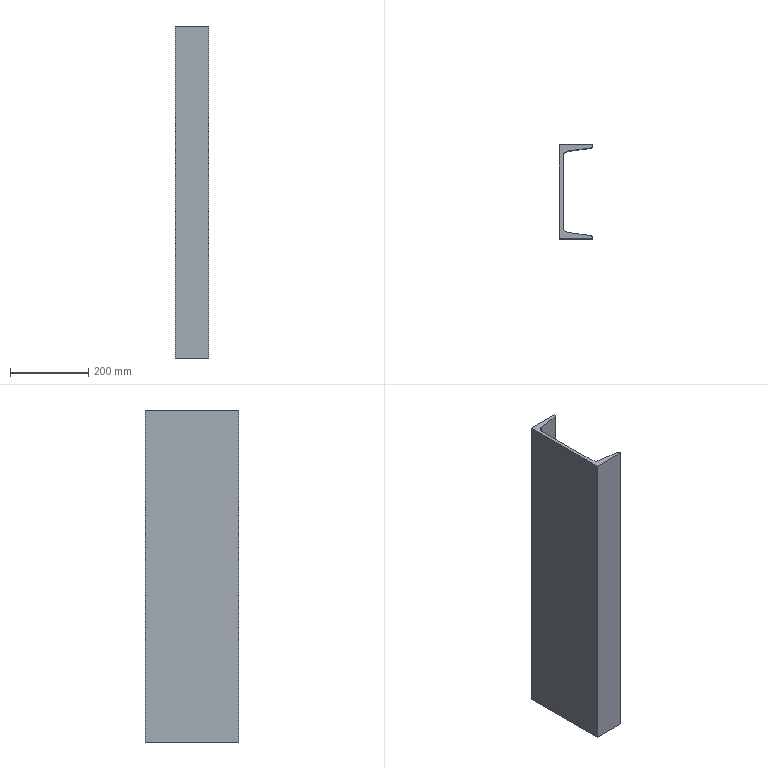Part | SolidWorks | features Extrusion 1 | 1 solid | 14 faces | box 85 x 240 x 850 mm | volume 3553986 mm3 | plane 10 | cylinder 4 | commonest cylinder face diameters 13 x2 26 x2
STEP:
#1=CARTESIAN_POINT('',(0.,-1.377,0.));
#2=VERTEX_POINT('',#1);
#3=CARTESIAN_POINT('',(0.,0.,0.));
#4=VERTEX_POINT('',#3);
#5=CARTESIAN_POINT('',(0.,-1.377,0.));
#6=DIRECTION('',(0.,1.,0.));
#7=VECTOR('',#6,1000.);
#8=LINE('',#5,#7);
#9=EDGE_CURVE('',#2,#4,#8,.T.);
#10=ORIENTED_EDGE('',*,*,#9,.T.);
#11=CARTESIAN_POINT('',(0.,0.,850.));
#12=VERTEX_POINT('',#11);
#13=CARTESIAN_POINT('',(0.,0.,850.));
#14=DIRECTION('',(0.,0.,-1.));
#15=VECTOR('',#14,1000.);
#16=LINE('',#13,#15);
#17=EDGE_CURVE('',#12,#4,#16,.T.);
#18=ORIENTED_EDGE('',*,*,#17,.F.);
#19=CARTESIAN_POINT('',(0.,-1.377,850.));
#20=VERTEX_POINT('',#19);
#21=CARTESIAN_POINT('',(0.,-1.377,850.));
#22=DIRECTION('',(0.,1.,0.));
#23=VECTOR('',#22,1000.);
#24=LINE('',#21,#23);
#25=EDGE_CURVE('',#20,#12,#24,.T.);
#26=ORIENTED_EDGE('',*,*,#25,.F.);
#27=CARTESIAN_POINT('',(0.,-1.377,850.));
#28=DIRECTION('',(0.,0.,-1.));
#29=VECTOR('',#28,1000.);
#30=LINE('',#27,#29);
#31=EDGE_CURVE('',#20,#2,#30,.T.);
#32=ORIENTED_EDGE('',*,*,#31,.T.);
#33=EDGE_LOOP('',(#10,#18,#26,#32));
#34=FACE_OUTER_BOUND('',#33,.T.);
#35=CARTESIAN_POINT('',(0.,-1.377,850.));
#36=DIRECTION('',(-1.,0.,0.));
#37=DIRECTION('',(0.,0.,1.));
#38=AXIS2_PLACEMENT_3D('',#35,#36,#37);
#39=PLANE('',#38);
#40=ADVANCED_FACE('',(#34),#39,.F.);
#41=CARTESIAN_POINT('',(-85.,0.,0.));
#42=VERTEX_POINT('',#41);
#43=CARTESIAN_POINT('',(0.,0.,0.));
#44=DIRECTION('',(-1.,0.,0.));
#45=VECTOR('',#44,1000.);
#46=LINE('',#43,#45);
#47=EDGE_CURVE('',#4,#42,#46,.T.);
#48=ORIENTED_EDGE('',*,*,#47,.T.);
#49=CARTESIAN_POINT('',(-85.,0.,850.));
#50=VERTEX_POINT('',#49);
#51=CARTESIAN_POINT('',(-85.,0.,850.));
#52=DIRECTION('',(0.,0.,-1.));
#53=VECTOR('',#52,1000.);
#54=LINE('',#51,#53);
#55=EDGE_CURVE('',#50,#42,#54,.T.);
#56=ORIENTED_EDGE('',*,*,#55,.F.);
#57=CARTESIAN_POINT('',(0.,0.,850.));
#58=DIRECTION('',(-1.,0.,0.));
#59=VECTOR('',#58,1000.);
#60=LINE('',#57,#59);
#61=EDGE_CURVE('',#12,#50,#60,.T.);
#62=ORIENTED_EDGE('',*,*,#61,.F.);
#63=ORIENTED_EDGE('',*,*,#17,.T.);
#64=EDGE_LOOP('',(#48,#56,#62,#63));
#65=FACE_OUTER_BOUND('',#64,.T.);
#66=CARTESIAN_POINT('',(0.,0.,850.));
#67=DIRECTION('',(0.,-1.,0.));
#68=DIRECTION('',(1.,0.,0.));
#69=AXIS2_PLACEMENT_3D('',#66,#67,#68);
#70=PLANE('',#69);
#71=ADVANCED_FACE('',(#65),#70,.F.);
#72=CARTESIAN_POINT('',(-85.,-240.,0.));
#73=VERTEX_POINT('',#72);
#74=CARTESIAN_POINT('',(-85.,0.,0.));
#75=DIRECTION('',(0.,-1.,0.));
#76=VECTOR('',#75,1000.);
#77=LINE('',#74,#76);
#78=EDGE_CURVE('',#42,#73,#77,.T.);
#79=ORIENTED_EDGE('',*,*,#78,.T.);
#80=CARTESIAN_POINT('',(-85.,-240.,850.));
#81=VERTEX_POINT('',#80);
#82=CARTESIAN_POINT('',(-85.,-240.,850.));
#83=DIRECTION('',(0.,0.,-1.));
#84=VECTOR('',#83,1000.);
#85=LINE('',#82,#84);
#86=EDGE_CURVE('',#81,#73,#85,.T.);
#87=ORIENTED_EDGE('',*,*,#86,.F.);
#88=CARTESIAN_POINT('',(-85.,0.,850.));
#89=DIRECTION('',(0.,-1.,0.));
#90=VECTOR('',#89,1000.);
#91=LINE('',#88,#90);
#92=EDGE_CURVE('',#50,#81,#91,.T.);
#93=ORIENTED_EDGE('',*,*,#92,.F.);
#94=ORIENTED_EDGE('',*,*,#55,.T.);
#95=EDGE_LOOP('',(#79,#87,#93,#94));
#96=FACE_OUTER_BOUND('',#95,.T.);
#97=CARTESIAN_POINT('',(-85.,0.,850.));
#98=DIRECTION('',(1.,0.,0.));
#99=DIRECTION('',(0.,1.,0.));
#100=AXIS2_PLACEMENT_3D('',#97,#98,#99);
#101=PLANE('',#100);
#102=ADVANCED_FACE('',(#96),#101,.F.);
#103=CARTESIAN_POINT('',(0.,-240.,0.));
#104=VERTEX_POINT('',#103);
#105=CARTESIAN_POINT('',(-85.,-240.,0.));
#106=DIRECTION('',(1.,0.,0.));
#107=VECTOR('',#106,1000.);
#108=LINE('',#105,#107);
#109=EDGE_CURVE('',#73,#104,#108,.T.);
#110=ORIENTED_EDGE('',*,*,#109,.T.);
#111=CARTESIAN_POINT('',(0.,-240.,850.));
#112=VERTEX_POINT('',#111);
#113=CARTESIAN_POINT('',(0.,-240.,850.));
#114=DIRECTION('',(0.,0.,-1.));
#115=VECTOR('',#114,1000.);
#116=LINE('',#113,#115);
#117=EDGE_CURVE('',#112,#104,#116,.T.);
#118=ORIENTED_EDGE('',*,*,#117,.F.);
#119=CARTESIAN_POINT('',(-85.,-240.,850.));
#120=DIRECTION('',(1.,0.,0.));
#121=VECTOR('',#120,1000.);
#122=LINE('',#119,#121);
#123=EDGE_CURVE('',#81,#112,#122,.T.);
#124=ORIENTED_EDGE('',*,*,#123,.F.);
#125=ORIENTED_EDGE('',*,*,#86,.T.);
#126=EDGE_LOOP('',(#110,#118,#124,#125));
#127=FACE_OUTER_BOUND('',#126,.T.);
#128=CARTESIAN_POINT('',(-85.,-240.,850.));
#129=DIRECTION('',(0.,1.,0.));
#130=DIRECTION('',(0.,0.,1.));
#131=AXIS2_PLACEMENT_3D('',#128,#129,#130);
#132=PLANE('',#131);
#133=ADVANCED_FACE('',(#127),#132,.F.);
#134=CARTESIAN_POINT('',(0.,-238.623,0.));
#135=VERTEX_POINT('',#134);
#136=CARTESIAN_POINT('',(0.,-240.,0.));
#137=DIRECTION('',(0.,1.,0.));
#138=VECTOR('',#137,1000.);
#139=LINE('',#136,#138);
#140=EDGE_CURVE('',#104,#135,#139,.T.);
#141=ORIENTED_EDGE('',*,*,#140,.T.);
#142=CARTESIAN_POINT('',(0.,-238.623,850.));
#143=VERTEX_POINT('',#142);
#144=CARTESIAN_POINT('',(0.,-238.623,850.));
#145=DIRECTION('',(0.,0.,-1.));
#146=VECTOR('',#145,1000.);
#147=LINE('',#144,#146);
#148=EDGE_CURVE('',#143,#135,#147,.T.);
#149=ORIENTED_EDGE('',*,*,#148,.F.);
#150=CARTESIAN_POINT('',(0.,-240.,850.));
#151=DIRECTION('',(0.,1.,0.));
#152=VECTOR('',#151,1000.);
#153=LINE('',#150,#152);
#154=EDGE_CURVE('',#112,#143,#153,.T.);
#155=ORIENTED_EDGE('',*,*,#154,.F.);
#156=ORIENTED_EDGE('',*,*,#117,.T.);
#157=EDGE_LOOP('',(#141,#149,#155,#156));
#158=FACE_OUTER_BOUND('',#157,.T.);
#159=CARTESIAN_POINT('',(0.,-240.,850.));
#160=DIRECTION('',(-1.,0.,0.));
#161=DIRECTION('',(0.,-1.,0.));
#162=AXIS2_PLACEMENT_3D('',#159,#160,#161);
#163=PLANE('',#162);
#164=ADVANCED_FACE('',(#158),#163,.F.);
#165=CARTESIAN_POINT('',(-5.595,-232.187,0.));
#166=VERTEX_POINT('',#165);
#167=CARTESIAN_POINT('',(-6.5,-238.623,0.));
#168=DIRECTION('',(0.,0.,1.));
#169=DIRECTION('',(1.,0.,0.));
#170=AXIS2_PLACEMENT_3D('',#167,#168,#169);
#171=CIRCLE('',#170,6.5);
#172=EDGE_CURVE('',#135,#166,#171,.T.);
#173=ORIENTED_EDGE('',*,*,#172,.T.);
#174=CARTESIAN_POINT('',(-5.595,-232.187,850.));
#175=VERTEX_POINT('',#174);
#176=CARTESIAN_POINT('',(-5.595,-232.187,850.));
#177=DIRECTION('',(0.,0.,-1.));
#178=VECTOR('',#177,1000.);
#179=LINE('',#176,#178);
#180=EDGE_CURVE('',#175,#166,#179,.T.);
#181=ORIENTED_EDGE('',*,*,#180,.F.);
#182=CARTESIAN_POINT('',(-6.5,-238.623,850.));
#183=DIRECTION('',(0.,0.,1.));
#184=DIRECTION('',(1.,0.,0.));
#185=AXIS2_PLACEMENT_3D('',#182,#183,#184);
#186=CIRCLE('',#185,6.5);
#187=EDGE_CURVE('',#143,#175,#186,.T.);
#188=ORIENTED_EDGE('',*,*,#187,.F.);
#189=ORIENTED_EDGE('',*,*,#148,.T.);
#190=EDGE_LOOP('',(#173,#181,#188,#189));
#191=FACE_OUTER_BOUND('',#190,.T.);
#192=CARTESIAN_POINT('',(-6.5,-238.623,850.));
#193=DIRECTION('',(0.,0.,-1.));
#194=DIRECTION('',(-1.,0.,0.));
#195=AXIS2_PLACEMENT_3D('',#192,#193,#194);
#196=CYLINDRICAL_SURFACE('',#195,6.5);
#197=ADVANCED_FACE('',(#191),#196,.T.);
#198=CARTESIAN_POINT('',(-64.309,-223.935,0.));
#199=VERTEX_POINT('',#198);
#200=CARTESIAN_POINT('',(-5.595,-232.187,0.));
#201=DIRECTION('',(-0.9903,0.1392,0.));
#202=VECTOR('',#201,1000.);
#203=LINE('',#200,#202);
#204=EDGE_CURVE('',#166,#199,#203,.T.);
#205=ORIENTED_EDGE('',*,*,#204,.T.);
#206=CARTESIAN_POINT('',(-64.309,-223.935,850.));
#207=VERTEX_POINT('',#206);
#208=CARTESIAN_POINT('',(-64.309,-223.935,850.));
#209=DIRECTION('',(0.,0.,-1.));
#210=VECTOR('',#209,1000.);
#211=LINE('',#208,#210);
#212=EDGE_CURVE('',#207,#199,#211,.T.);
#213=ORIENTED_EDGE('',*,*,#212,.F.);
#214=CARTESIAN_POINT('',(-5.595,-232.187,850.));
#215=DIRECTION('',(-0.9903,0.1392,0.));
#216=VECTOR('',#215,1000.);
#217=LINE('',#214,#216);
#218=EDGE_CURVE('',#175,#207,#217,.T.);
#219=ORIENTED_EDGE('',*,*,#218,.F.);
#220=ORIENTED_EDGE('',*,*,#180,.T.);
#221=EDGE_LOOP('',(#205,#213,#219,#220));
#222=FACE_OUTER_BOUND('',#221,.T.);
#223=CARTESIAN_POINT('',(-5.595,-232.187,850.));
#224=DIRECTION('',(-0.1392,-0.9903,0.));
#225=DIRECTION('',(0.9903,-0.1392,0.));
#226=AXIS2_PLACEMENT_3D('',#223,#224,#225);
#227=PLANE('',#226);
#228=ADVANCED_FACE('',(#222),#227,.F.);
#229=CARTESIAN_POINT('',(-75.5,-211.061,0.));
#230=VERTEX_POINT('',#229);
#231=CARTESIAN_POINT('',(-62.5,-211.061,0.));
#232=DIRECTION('',(0.,0.,-1.));
#233=DIRECTION('',(-1.,0.,0.));
#234=AXIS2_PLACEMENT_3D('',#231,#232,#233);
#235=CIRCLE('',#234,13.);
#236=EDGE_CURVE('',#199,#230,#235,.T.);
#237=ORIENTED_EDGE('',*,*,#236,.T.);
#238=CARTESIAN_POINT('',(-75.5,-211.061,850.));
#239=VERTEX_POINT('',#238);
#240=CARTESIAN_POINT('',(-75.5,-211.061,850.));
#241=DIRECTION('',(0.,0.,-1.));
#242=VECTOR('',#241,1000.);
#243=LINE('',#240,#242);
#244=EDGE_CURVE('',#239,#230,#243,.T.);
#245=ORIENTED_EDGE('',*,*,#244,.F.);
#246=CARTESIAN_POINT('',(-62.5,-211.061,850.));
#247=DIRECTION('',(0.,0.,-1.));
#248=DIRECTION('',(-1.,0.,0.));
#249=AXIS2_PLACEMENT_3D('',#246,#247,#248);
#250=CIRCLE('',#249,13.);
#251=EDGE_CURVE('',#207,#239,#250,.T.);
#252=ORIENTED_EDGE('',*,*,#251,.F.);
#253=ORIENTED_EDGE('',*,*,#212,.T.);
#254=EDGE_LOOP('',(#237,#245,#252,#253));
#255=FACE_OUTER_BOUND('',#254,.T.);
#256=CARTESIAN_POINT('',(-62.5,-211.061,850.));
#257=DIRECTION('',(0.,0.,-1.));
#258=DIRECTION('',(-1.,0.,0.));
#259=AXIS2_PLACEMENT_3D('',#256,#257,#258);
#260=CYLINDRICAL_SURFACE('',#259,13.);
#261=ADVANCED_FACE('',(#255),#260,.F.);
#262=CARTESIAN_POINT('',(-75.5,-28.939,0.));
#263=VERTEX_POINT('',#262);
#264=CARTESIAN_POINT('',(-75.5,-211.061,0.));
#265=DIRECTION('',(0.,1.,0.));
#266=VECTOR('',#265,1000.);
#267=LINE('',#264,#266);
#268=EDGE_CURVE('',#230,#263,#267,.T.);
#269=ORIENTED_EDGE('',*,*,#268,.T.);
#270=CARTESIAN_POINT('',(-75.5,-28.939,850.));
#271=VERTEX_POINT('',#270);
#272=CARTESIAN_POINT('',(-75.5,-28.939,850.));
#273=DIRECTION('',(0.,0.,-1.));
#274=VECTOR('',#273,1000.);
#275=LINE('',#272,#274);
#276=EDGE_CURVE('',#271,#263,#275,.T.);
#277=ORIENTED_EDGE('',*,*,#276,.F.);
#278=CARTESIAN_POINT('',(-75.5,-211.061,850.));
#279=DIRECTION('',(0.,1.,0.));
#280=VECTOR('',#279,1000.);
#281=LINE('',#278,#280);
#282=EDGE_CURVE('',#239,#271,#281,.T.);
#283=ORIENTED_EDGE('',*,*,#282,.F.);
#284=ORIENTED_EDGE('',*,*,#244,.T.);
#285=EDGE_LOOP('',(#269,#277,#283,#284));
#286=FACE_OUTER_BOUND('',#285,.T.);
#287=CARTESIAN_POINT('',(-75.5,-211.061,850.));
#288=DIRECTION('',(-1.,0.,0.));
#289=DIRECTION('',(0.,0.,1.));
#290=AXIS2_PLACEMENT_3D('',#287,#288,#289);
#291=PLANE('',#290);
#292=ADVANCED_FACE('',(#286),#291,.F.);
#293=CARTESIAN_POINT('',(-64.309,-16.065,0.));
#294=VERTEX_POINT('',#293);
#295=CARTESIAN_POINT('',(-62.5,-28.939,0.));
#296=DIRECTION('',(0.,0.,-1.));
#297=DIRECTION('',(-1.,0.,0.));
#298=AXIS2_PLACEMENT_3D('',#295,#296,#297);
#299=CIRCLE('',#298,13.);
#300=EDGE_CURVE('',#263,#294,#299,.T.);
#301=ORIENTED_EDGE('',*,*,#300,.T.);
#302=CARTESIAN_POINT('',(-64.309,-16.065,850.));
#303=VERTEX_POINT('',#302);
#304=CARTESIAN_POINT('',(-64.309,-16.065,850.));
#305=DIRECTION('',(0.,0.,-1.));
#306=VECTOR('',#305,1000.);
#307=LINE('',#304,#306);
#308=EDGE_CURVE('',#303,#294,#307,.T.);
#309=ORIENTED_EDGE('',*,*,#308,.F.);
#310=CARTESIAN_POINT('',(-62.5,-28.939,850.));
#311=DIRECTION('',(0.,0.,-1.));
#312=DIRECTION('',(-1.,0.,0.));
#313=AXIS2_PLACEMENT_3D('',#310,#311,#312);
#314=CIRCLE('',#313,13.);
#315=EDGE_CURVE('',#271,#303,#314,.T.);
#316=ORIENTED_EDGE('',*,*,#315,.F.);
#317=ORIENTED_EDGE('',*,*,#276,.T.);
#318=EDGE_LOOP('',(#301,#309,#316,#317));
#319=FACE_OUTER_BOUND('',#318,.T.);
#320=CARTESIAN_POINT('',(-62.5,-28.939,850.));
#321=DIRECTION('',(0.,0.,-1.));
#322=DIRECTION('',(-1.,0.,0.));
#323=AXIS2_PLACEMENT_3D('',#320,#321,#322);
#324=CYLINDRICAL_SURFACE('',#323,13.);
#325=ADVANCED_FACE('',(#319),#324,.F.);
#326=CARTESIAN_POINT('',(-5.595,-7.813,0.));
#327=VERTEX_POINT('',#326);
#328=CARTESIAN_POINT('',(-64.309,-16.065,0.));
#329=DIRECTION('',(0.9903,0.1392,0.));
#330=VECTOR('',#329,1000.);
#331=LINE('',#328,#330);
#332=EDGE_CURVE('',#294,#327,#331,.T.);
#333=ORIENTED_EDGE('',*,*,#332,.T.);
#334=CARTESIAN_POINT('',(-5.595,-7.813,850.));
#335=VERTEX_POINT('',#334);
#336=CARTESIAN_POINT('',(-5.595,-7.813,850.));
#337=DIRECTION('',(0.,0.,-1.));
#338=VECTOR('',#337,1000.);
#339=LINE('',#336,#338);
#340=EDGE_CURVE('',#335,#327,#339,.T.);
#341=ORIENTED_EDGE('',*,*,#340,.F.);
#342=CARTESIAN_POINT('',(-64.309,-16.065,850.));
#343=DIRECTION('',(0.9903,0.1392,0.));
#344=VECTOR('',#343,1000.);
#345=LINE('',#342,#344);
#346=EDGE_CURVE('',#303,#335,#345,.T.);
#347=ORIENTED_EDGE('',*,*,#346,.F.);
#348=ORIENTED_EDGE('',*,*,#308,.T.);
#349=EDGE_LOOP('',(#333,#341,#347,#348));
#350=FACE_OUTER_BOUND('',#349,.T.);
#351=CARTESIAN_POINT('',(-64.309,-16.065,850.));
#352=DIRECTION('',(-0.1392,0.9903,0.));
#353=DIRECTION('',(-0.9903,-0.1392,0.));
#354=AXIS2_PLACEMENT_3D('',#351,#352,#353);
#355=PLANE('',#354);
#356=ADVANCED_FACE('',(#350),#355,.F.);
#357=CARTESIAN_POINT('',(-6.5,-1.377,0.));
#358=DIRECTION('',(0.,0.,1.));
#359=DIRECTION('',(1.,0.,0.));
#360=AXIS2_PLACEMENT_3D('',#357,#358,#359);
#361=CIRCLE('',#360,6.5);
#362=EDGE_CURVE('',#327,#2,#361,.T.);
#363=ORIENTED_EDGE('',*,*,#362,.T.);
#364=ORIENTED_EDGE('',*,*,#31,.F.);
#365=CARTESIAN_POINT('',(-6.5,-1.377,850.));
#366=DIRECTION('',(0.,0.,1.));
#367=DIRECTION('',(1.,0.,0.));
#368=AXIS2_PLACEMENT_3D('',#365,#366,#367);
#369=CIRCLE('',#368,6.5);
#370=EDGE_CURVE('',#335,#20,#369,.T.);
#371=ORIENTED_EDGE('',*,*,#370,.F.);
#372=ORIENTED_EDGE('',*,*,#340,.T.);
#373=EDGE_LOOP('',(#363,#364,#371,#372));
#374=FACE_OUTER_BOUND('',#373,.T.);
#375=CARTESIAN_POINT('',(-6.5,-1.377,850.));
#376=DIRECTION('',(0.,0.,-1.));
#377=DIRECTION('',(-1.,0.,0.));
#378=AXIS2_PLACEMENT_3D('',#375,#376,#377);
#379=CYLINDRICAL_SURFACE('',#378,6.5);
#380=ADVANCED_FACE('',(#374),#379,.T.);
#381=ORIENTED_EDGE('',*,*,#25,.T.);
#382=ORIENTED_EDGE('',*,*,#61,.T.);
#383=ORIENTED_EDGE('',*,*,#92,.T.);
#384=ORIENTED_EDGE('',*,*,#123,.T.);
#385=ORIENTED_EDGE('',*,*,#154,.T.);
#386=ORIENTED_EDGE('',*,*,#187,.T.);
#387=ORIENTED_EDGE('',*,*,#218,.T.);
#388=ORIENTED_EDGE('',*,*,#251,.T.);
#389=ORIENTED_EDGE('',*,*,#282,.T.);
#390=ORIENTED_EDGE('',*,*,#315,.T.);
#391=ORIENTED_EDGE('',*,*,#346,.T.);
#392=ORIENTED_EDGE('',*,*,#370,.T.);
#393=EDGE_LOOP('',(#381,#382,#383,#384,#385,#386,#387,#388,#389,#390,#391,#392));
#394=FACE_OUTER_BOUND('',#393,.T.);
#395=CARTESIAN_POINT('',(-6.5,-238.623,850.));
#396=DIRECTION('',(0.,0.,1.));
#397=DIRECTION('',(1.,0.,0.));
#398=AXIS2_PLACEMENT_3D('',#395,#396,#397);
#399=PLANE('',#398);
#400=ADVANCED_FACE('',(#394),#399,.T.);
#401=ORIENTED_EDGE('',*,*,#9,.F.);
#402=ORIENTED_EDGE('',*,*,#362,.F.);
#403=ORIENTED_EDGE('',*,*,#332,.F.);
#404=ORIENTED_EDGE('',*,*,#300,.F.);
#405=ORIENTED_EDGE('',*,*,#268,.F.);
#406=ORIENTED_EDGE('',*,*,#236,.F.);
#407=ORIENTED_EDGE('',*,*,#204,.F.);
#408=ORIENTED_EDGE('',*,*,#172,.F.);
#409=ORIENTED_EDGE('',*,*,#140,.F.);
#410=ORIENTED_EDGE('',*,*,#109,.F.);
#411=ORIENTED_EDGE('',*,*,#78,.F.);
#412=ORIENTED_EDGE('',*,*,#47,.F.);
#413=EDGE_LOOP('',(#401,#402,#403,#404,#405,#406,#407,#408,#409,#410,#411,#412));
#414=FACE_OUTER_BOUND('',#413,.T.);
#415=CARTESIAN_POINT('',(-6.5,-238.623,0.));
#416=DIRECTION('',(0.,0.,1.));
#417=DIRECTION('',(1.,0.,0.));
#418=AXIS2_PLACEMENT_3D('',#415,#416,#417);
#419=PLANE('',#418);
#420=ADVANCED_FACE('',(#414),#419,.F.);
#421=CLOSED_SHELL('',(#40,#71,#102,#133,#164,#197,#228,#261,#292,#325,#356,#380,#400,#420));
#422=MANIFOLD_SOLID_BREP('',#421);
#423=CARTESIAN_POINT('',(0.,0.,0.));
#424=DIRECTION('',(0.,0.,1.));
#425=DIRECTION('',(1.,0.,0.));
#426=AXIS2_PLACEMENT_3D('',#423,#424,#425);
#427=(LENGTH_UNIT()NAMED_UNIT(*)SI_UNIT(.MILLI.,.METRE.));
#428=UNCERTAINTY_MEASURE_WITH_UNIT(LENGTH_MEASURE(0.00001),#427,'','');
#429=(NAMED_UNIT(*)PLANE_ANGLE_UNIT()SI_UNIT($,.RADIAN.));
#430=(NAMED_UNIT(*)SI_UNIT($,.STERADIAN.)SOLID_ANGLE_UNIT());
#431=(GEOMETRIC_REPRESENTATION_CONTEXT(3)GLOBAL_UNCERTAINTY_ASSIGNED_CONTEXT((#428))GLOBAL_UNIT_ASSIGNED_CONTEXT((#427,#429,#430))REPRESENTATION_CONTEXT('',''));
#432=ADVANCED_BREP_SHAPE_REPRESENTATION('',(#422,#426),#431);